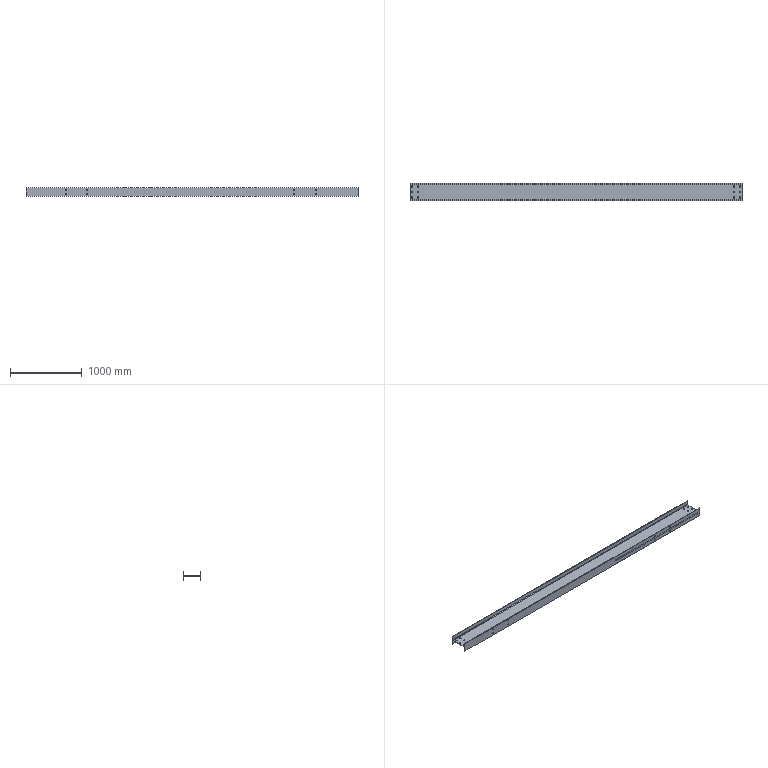Part | STEP file | 粉仓主梁4主体_Default<As Machined> | 1 solid | 58 faces | box 4620 x 250 x 125 mm | volume 17048565 mm3 | cylinder 44 | plane 14 | commonest cylinder face diameters 19 x24 15 x16 16 x4